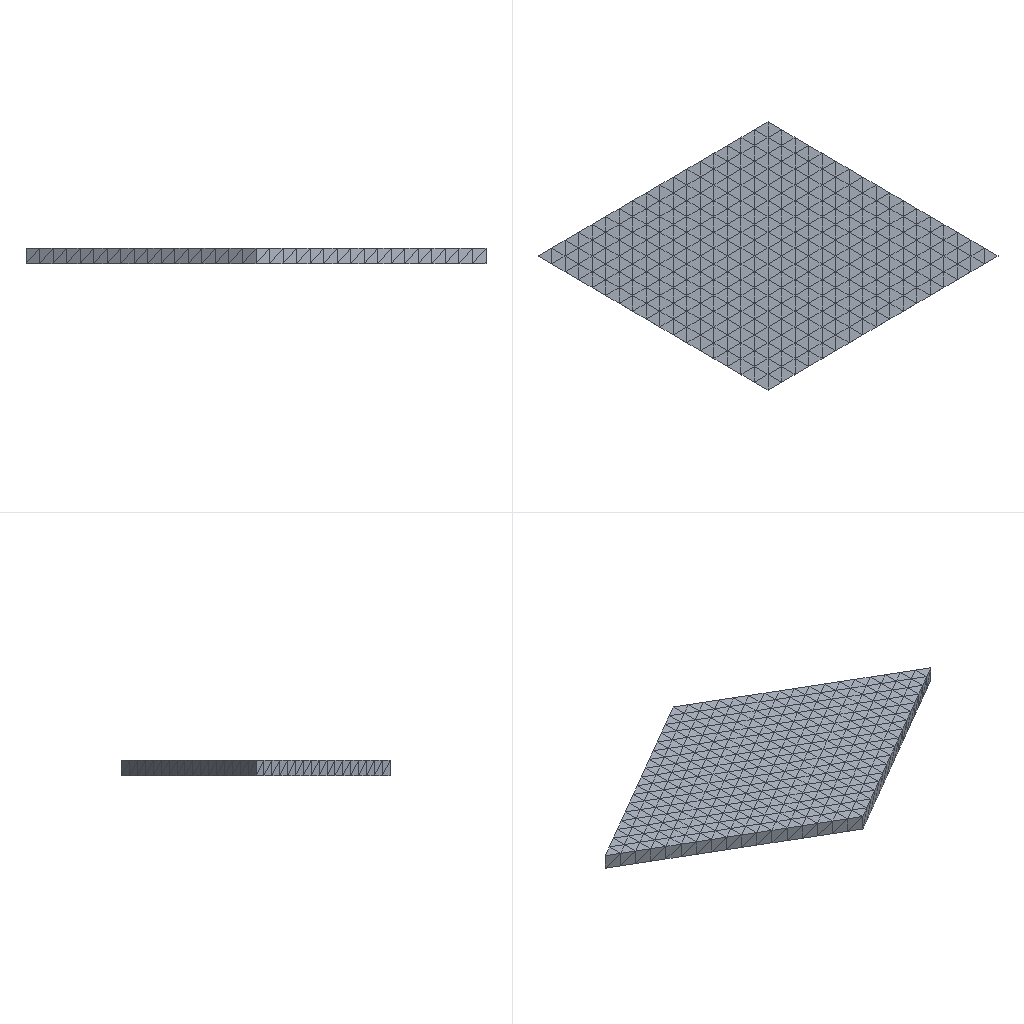Simulation study | abaqus
Notes in the study folder:
20 rhombus plate
job_status=None
Umax_mm=0.0216106
S_Mises_max_MPa=109.41
Set-up summary:
category,name,step,type,value,unit,region
solver,abaqus,,Abaqus/CAE 2024
units,mm-N-s-tonne (MPa),,inferred,E=210000 density=7.85e-09
analysis,Step-1,,static,time_period=1
mesh,nodes,,,3675
mesh,elements,,,1734
element_type,C3D10,,,1734
material,Steel,,E,210000
material,Steel,,nu,0.3
material,Steel,,density,7.85e-09
section,Steel,,solid section,,,_PickedSet2
load,P,Step-1,pressure,0.1,,PRESS
bc,BC,Step-1,encastre,[dofs=ENCASTRE],,FIXED
Abaqus input file, long lists of numbers shortened:
*Heading
** Job name: deck Model name: M20
** Generated by: Abaqus/CAE 2024
*Preprint, echo=NO, model=NO, history=NO, contact=NO
**
** PARTS
**
*Part, name=P
*Node
      1,           0.,         -35.,           4.
      2,         -60.,           0.,           4.
** (3673 more lines like these left out)
*Element, type=C3D10
   1,  624,  623,  281,  282,  651,  650,  649,  653,  652,  654
   2,  622,  298,  297,  282,  657,  656,  655,  659,  658,  660
** (1732 more lines like these left out)
*Nset, nset=_PickedSet2, internal, generate
    1,  3675,     1
*Elset, elset=_PickedSet2, internal, generate
    1,  1734,     1
** Section: Sec
*Solid Section, elset=_PickedSet2, material=Steel
,
*End Part
**
**
** ASSEMBLY
**
*Assembly, name=Assembly
**
*Instance, name=I, part=P
*End Instance
**
*Nset, nset=FIXED, instance=I
 3, 4, 6, 7
*Elset, elset=_PRESS_S1, internal, instance=I
    3,   11,   16,   20,   26,   48,   61,   69,   81,   84,   94,  100,  102,  103,  116,  122
  126,  132,  133,  135,  136,  165,  170,  176,  184,  198,  203,  204,  217,  227,  234,  237
** (10 more lines like these left out)
*Elset, elset=_PRESS_S2, internal, instance=I
    5,    7,   15,   30,   31,   32,   34,   39,   63,   67,   82,   93,   95,   98,  124,  134
  137,  148,  152,  153,  156,  157,  189,  192,  199,  201,  202,  208,  213,  223,  235,  240
** (14 more lines like these left out)
*Elset, elset=_PRESS_S4, internal, instance=I
   18,   24,   36,   42,   43,   51,   55,   58,   59,   64,   66,   77,   89,   90,   91,  105
  110,  119,  121,  123,  127,  128,  140,  169,  175,  193,  220,  225,  247,  276,  295,  298
** (7 more lines like these left out)
*Elset, elset=_PRESS_S3, internal, instance=I
  969, 1323, 1456, 1514, 1528
*Surface, type=ELEMENT, name=PRESS
_PRESS_S1, S1
_PRESS_S2, S2
_PRESS_S4, S4
_PRESS_S3, S3
*End Assembly
**
** MATERIALS
**
*Material, name=Steel
*Density
 7.85e-09,
*Elastic
210000., 0.3
** ----------------------------------------------------------------
**
** STEP: Step-1
**
*Step, name=Step-1, nlgeom=NO
*Static
1., 1., 1e-05, 1.
**
** BOUNDARY CONDITIONS
**
** Name: BC Type: Symmetry/Antisymmetry/Encastre
*Boundary
FIXED, ENCASTRE
**
** LOADS
**
** Name: P   Type: Pressure
*Dsload
PRESS, P, 0.1
**
** OUTPUT REQUESTS
**
*Restart, write, frequency=0
**
** FIELD OUTPUT: F-Output-1
**
*Output, field, variable=PRESELECT
**
** HISTORY OUTPUT: H-Output-1
**
*Output, history, variable=PRESELECT
*End Step
Results summary:
result,odb.job_status,,,JOB_STATUS_COMPLETED_SUCCESSFULLY,"consistent, unstated (Abaqus has no unit system)"
result,steps[0].procedure,Step-1,,*STATIC,"consistent, unstated (Abaqus has no unit system)"
result,steps[0].time_period,Step-1,,1,"consistent, unstated (Abaqus has no unit system)"
result,steps[0].n_frames,Step-1,,2,"consistent, unstated (Abaqus has no unit system)"
result,steps[0].last_frame.id,Step-1,,1,"consistent, unstated (Abaqus has no unit system)"
result,steps[0].last_frame.value,Step-1,,1,"consistent, unstated (Abaqus has no unit system)"
result,steps[0].last_frame.description,Step-1,,Increment      1: Step Time =    1.000,"consistent, unstated (Abaqus has no unit system)"
result,steps[0].completed,Step-1,,True,"consistent, unstated (Abaqus has no unit system)"
result,steps[0].max_U_magnitude,Step-1,,0.02161,"consistent, unstated (Abaqus has no unit system)"
result,steps[0].max_S_mises,Step-1,,109.41,"consistent, unstated (Abaqus has no unit system)"
result,steps[0].RF_sum[1],Step-1,,-1.52588e-05,"consistent, unstated (Abaqus has no unit system)"
result,steps[0].RF_sum[2],Step-1,,1.19209e-06,"consistent, unstated (Abaqus has no unit system)"
result,steps[0].RF_sum[3],Step-1,,420,"consistent, unstated (Abaqus has no unit system)"
result,steps[1].procedure,Step-1,,*STATIC,"consistent, unstated (Abaqus has no unit system)"
result,steps[1].time_period,Step-1,,1,"consistent, unstated (Abaqus has no unit system)"
result,steps[1].n_frames,Step-1,,2,"consistent, unstated (Abaqus has no unit system)"
result,steps[1].last_frame.id,Step-1,,1,"consistent, unstated (Abaqus has no unit system)"
result,steps[1].last_frame.value,Step-1,,1,"consistent, unstated (Abaqus has no unit system)"
result,steps[1].last_frame.description,Step-1,,Increment      1: Step Time =    1.000,"consistent, unstated (Abaqus has no unit system)"
result,steps[1].completed,Step-1,,True,"consistent, unstated (Abaqus has no unit system)"
result,steps[1].max_U_magnitude,Step-1,,0.02161,"consistent, unstated (Abaqus has no unit system)"
result,steps[1].max_S_mises,Step-1,,109.41,"consistent, unstated (Abaqus has no unit system)"
result,steps[1].RF_sum[1],Step-1,,-1.52588e-05,"consistent, unstated (Abaqus has no unit system)"
result,steps[1].RF_sum[2],Step-1,,1.19209e-06,"consistent, unstated (Abaqus has no unit system)"
result,steps[1].RF_sum[3],Step-1,,420,"consistent, unstated (Abaqus has no unit system)"